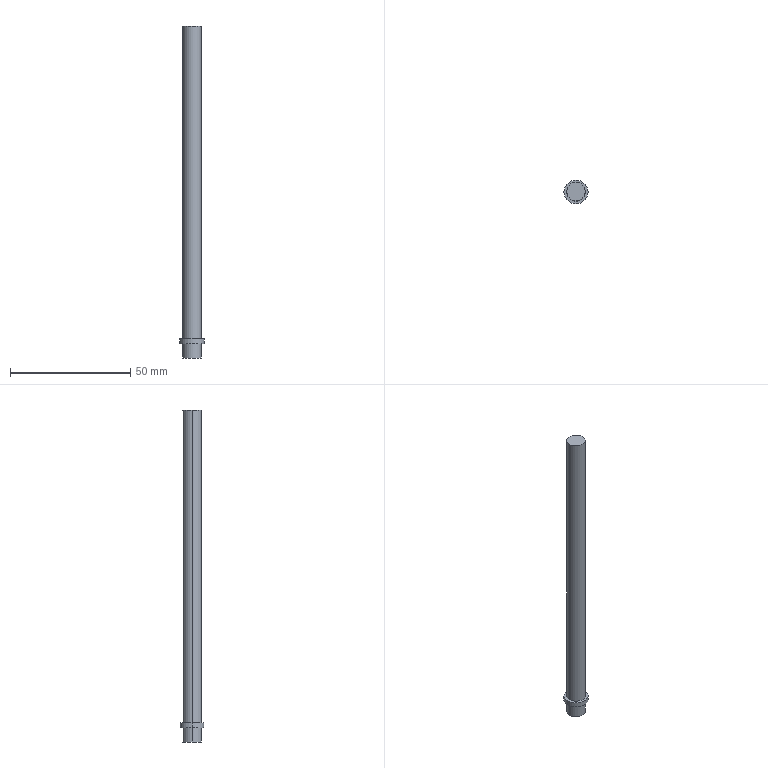Part | SolidWorks | features BaseBody 1 | 1 solid | 10 faces | box 10 x 10 x 138 mm | volume 6490 mm3 | cylinder 6 | plane 4 | commonest cylinder face diameters 7.7 x4 10 x2
STEP:
#1=CARTESIAN_POINT('',(-3.85,0.,-8.));
#2=VERTEX_POINT('',#1);
#3=CARTESIAN_POINT('',(3.85,0.,-8.));
#4=VERTEX_POINT('',#3);
#5=CARTESIAN_POINT('',(0.,0.,-8.));
#6=DIRECTION('',(0.,0.,-1.));
#7=DIRECTION('',(-1.,0.,0.));
#8=AXIS2_PLACEMENT_3D('',#5,#6,#7);
#9=CIRCLE('',#8,3.85);
#10=EDGE_CURVE('',#2,#4,#9,.T.);
#11=ORIENTED_EDGE('',*,*,#10,.F.);
#12=CARTESIAN_POINT('',(-3.85,0.,-2.));
#13=VERTEX_POINT('',#12);
#14=CARTESIAN_POINT('',(-3.85,0.,-8.));
#15=DIRECTION('',(0.,0.,1.));
#16=VECTOR('',#15,1000.);
#17=LINE('',#14,#16);
#18=EDGE_CURVE('',#2,#13,#17,.T.);
#19=ORIENTED_EDGE('',*,*,#18,.T.);
#20=CARTESIAN_POINT('',(3.85,0.,-2.));
#21=VERTEX_POINT('',#20);
#22=CARTESIAN_POINT('',(0.,0.,-2.));
#23=DIRECTION('',(0.,0.,-1.));
#24=DIRECTION('',(-1.,0.,0.));
#25=AXIS2_PLACEMENT_3D('',#22,#23,#24);
#26=CIRCLE('',#25,3.85);
#27=EDGE_CURVE('',#13,#21,#26,.T.);
#28=ORIENTED_EDGE('',*,*,#27,.T.);
#29=CARTESIAN_POINT('',(3.85,0.,-8.));
#30=DIRECTION('',(0.,0.,1.));
#31=VECTOR('',#30,1000.);
#32=LINE('',#29,#31);
#33=EDGE_CURVE('',#4,#21,#32,.T.);
#34=ORIENTED_EDGE('',*,*,#33,.F.);
#35=EDGE_LOOP('',(#11,#19,#28,#34));
#36=FACE_OUTER_BOUND('',#35,.T.);
#37=CARTESIAN_POINT('',(0.,0.,-8.));
#38=DIRECTION('',(0.,0.,1.));
#39=DIRECTION('',(1.,0.,0.));
#40=AXIS2_PLACEMENT_3D('',#37,#38,#39);
#41=CYLINDRICAL_SURFACE('',#40,3.85);
#42=ADVANCED_FACE('',(#36),#41,.T.);
#43=CARTESIAN_POINT('',(-5.,0.,-2.));
#44=VERTEX_POINT('',#43);
#45=CARTESIAN_POINT('',(5.,0.,-2.));
#46=VERTEX_POINT('',#45);
#47=CARTESIAN_POINT('',(0.,0.,-2.));
#48=DIRECTION('',(0.,0.,-1.));
#49=DIRECTION('',(-1.,0.,0.));
#50=AXIS2_PLACEMENT_3D('',#47,#48,#49);
#51=CIRCLE('',#50,5.);
#52=EDGE_CURVE('',#44,#46,#51,.T.);
#53=ORIENTED_EDGE('',*,*,#52,.F.);
#54=CARTESIAN_POINT('',(-5.,0.,0.));
#55=VERTEX_POINT('',#54);
#56=CARTESIAN_POINT('',(-5.,0.,-2.));
#57=DIRECTION('',(0.,0.,1.));
#58=VECTOR('',#57,1000.);
#59=LINE('',#56,#58);
#60=EDGE_CURVE('',#44,#55,#59,.T.);
#61=ORIENTED_EDGE('',*,*,#60,.T.);
#62=CARTESIAN_POINT('',(5.,0.,0.));
#63=VERTEX_POINT('',#62);
#64=CARTESIAN_POINT('',(0.,0.,0.));
#65=DIRECTION('',(0.,0.,-1.));
#66=DIRECTION('',(-1.,0.,0.));
#67=AXIS2_PLACEMENT_3D('',#64,#65,#66);
#68=CIRCLE('',#67,5.);
#69=EDGE_CURVE('',#55,#63,#68,.T.);
#70=ORIENTED_EDGE('',*,*,#69,.T.);
#71=CARTESIAN_POINT('',(5.,0.,-2.));
#72=DIRECTION('',(0.,0.,1.));
#73=VECTOR('',#72,1000.);
#74=LINE('',#71,#73);
#75=EDGE_CURVE('',#46,#63,#74,.T.);
#76=ORIENTED_EDGE('',*,*,#75,.F.);
#77=EDGE_LOOP('',(#53,#61,#70,#76));
#78=FACE_OUTER_BOUND('',#77,.T.);
#79=CARTESIAN_POINT('',(0.,0.,-2.));
#80=DIRECTION('',(0.,0.,1.));
#81=DIRECTION('',(1.,0.,0.));
#82=AXIS2_PLACEMENT_3D('',#79,#80,#81);
#83=CYLINDRICAL_SURFACE('',#82,5.);
#84=ADVANCED_FACE('',(#78),#83,.T.);
#85=CARTESIAN_POINT('',(3.85,0.,130.));
#86=VERTEX_POINT('',#85);
#87=CARTESIAN_POINT('',(-3.85,0.,130.));
#88=VERTEX_POINT('',#87);
#89=CARTESIAN_POINT('',(0.,0.,130.));
#90=DIRECTION('',(0.,0.,1.));
#91=DIRECTION('',(1.,0.,0.));
#92=AXIS2_PLACEMENT_3D('',#89,#90,#91);
#93=CIRCLE('',#92,3.85);
#94=EDGE_CURVE('',#86,#88,#93,.T.);
#95=ORIENTED_EDGE('',*,*,#94,.F.);
#96=CARTESIAN_POINT('',(3.85,0.,0.));
#97=VERTEX_POINT('',#96);
#98=CARTESIAN_POINT('',(3.85,0.,130.));
#99=DIRECTION('',(0.,0.,-1.));
#100=VECTOR('',#99,1000.);
#101=LINE('',#98,#100);
#102=EDGE_CURVE('',#86,#97,#101,.T.);
#103=ORIENTED_EDGE('',*,*,#102,.T.);
#104=CARTESIAN_POINT('',(-3.85,0.,0.));
#105=VERTEX_POINT('',#104);
#106=CARTESIAN_POINT('',(0.,0.,0.));
#107=DIRECTION('',(0.,0.,1.));
#108=DIRECTION('',(1.,0.,0.));
#109=AXIS2_PLACEMENT_3D('',#106,#107,#108);
#110=CIRCLE('',#109,3.85);
#111=EDGE_CURVE('',#97,#105,#110,.T.);
#112=ORIENTED_EDGE('',*,*,#111,.T.);
#113=CARTESIAN_POINT('',(-3.85,0.,130.));
#114=DIRECTION('',(0.,0.,-1.));
#115=VECTOR('',#114,1000.);
#116=LINE('',#113,#115);
#117=EDGE_CURVE('',#88,#105,#116,.T.);
#118=ORIENTED_EDGE('',*,*,#117,.F.);
#119=EDGE_LOOP('',(#95,#103,#112,#118));
#120=FACE_OUTER_BOUND('',#119,.T.);
#121=CARTESIAN_POINT('',(0.,0.,130.));
#122=DIRECTION('',(0.,0.,-1.));
#123=DIRECTION('',(-1.,0.,0.));
#124=AXIS2_PLACEMENT_3D('',#121,#122,#123);
#125=CYLINDRICAL_SURFACE('',#124,3.85);
#126=ADVANCED_FACE('',(#120),#125,.T.);
#127=CARTESIAN_POINT('',(0.,0.,-8.));
#128=DIRECTION('',(0.,0.,-1.));
#129=DIRECTION('',(-1.,0.,0.));
#130=AXIS2_PLACEMENT_3D('',#127,#128,#129);
#131=CIRCLE('',#130,3.85);
#132=EDGE_CURVE('',#4,#2,#131,.T.);
#133=ORIENTED_EDGE('',*,*,#132,.T.);
#134=ORIENTED_EDGE('',*,*,#10,.T.);
#135=EDGE_LOOP('',(#133,#134));
#136=FACE_OUTER_BOUND('',#135,.T.);
#137=CARTESIAN_POINT('',(0.,0.,-8.));
#138=DIRECTION('',(0.,0.,-1.));
#139=DIRECTION('',(0.,-1.,0.));
#140=AXIS2_PLACEMENT_3D('',#137,#138,#139);
#141=PLANE('',#140);
#142=ADVANCED_FACE('',(#136),#141,.T.);
#143=CARTESIAN_POINT('',(0.,0.,0.));
#144=DIRECTION('',(0.,0.,1.));
#145=DIRECTION('',(1.,0.,0.));
#146=AXIS2_PLACEMENT_3D('',#143,#144,#145);
#147=CIRCLE('',#146,3.85);
#148=EDGE_CURVE('',#105,#97,#147,.T.);
#149=ORIENTED_EDGE('',*,*,#148,.F.);
#150=ORIENTED_EDGE('',*,*,#111,.F.);
#151=EDGE_LOOP('',(#149,#150));
#152=FACE_BOUND('',#151,.T.);
#153=CARTESIAN_POINT('',(0.,0.,0.));
#154=DIRECTION('',(0.,0.,-1.));
#155=DIRECTION('',(-1.,0.,0.));
#156=AXIS2_PLACEMENT_3D('',#153,#154,#155);
#157=CIRCLE('',#156,5.);
#158=EDGE_CURVE('',#63,#55,#157,.T.);
#159=ORIENTED_EDGE('',*,*,#158,.F.);
#160=ORIENTED_EDGE('',*,*,#69,.F.);
#161=EDGE_LOOP('',(#159,#160));
#162=FACE_OUTER_BOUND('',#161,.T.);
#163=CARTESIAN_POINT('',(0.,0.,0.));
#164=DIRECTION('',(0.,0.,-1.));
#165=DIRECTION('',(0.,-1.,0.));
#166=AXIS2_PLACEMENT_3D('',#163,#164,#165);
#167=PLANE('',#166);
#168=ADVANCED_FACE('',(#152,#162),#167,.F.);
#169=CARTESIAN_POINT('',(0.,0.,-2.));
#170=DIRECTION('',(0.,0.,-1.));
#171=DIRECTION('',(-1.,0.,0.));
#172=AXIS2_PLACEMENT_3D('',#169,#170,#171);
#173=CIRCLE('',#172,3.85);
#174=EDGE_CURVE('',#21,#13,#173,.T.);
#175=ORIENTED_EDGE('',*,*,#174,.F.);
#176=ORIENTED_EDGE('',*,*,#27,.F.);
#177=EDGE_LOOP('',(#175,#176));
#178=FACE_BOUND('',#177,.T.);
#179=CARTESIAN_POINT('',(0.,0.,-2.));
#180=DIRECTION('',(0.,0.,-1.));
#181=DIRECTION('',(-1.,0.,0.));
#182=AXIS2_PLACEMENT_3D('',#179,#180,#181);
#183=CIRCLE('',#182,5.);
#184=EDGE_CURVE('',#46,#44,#183,.T.);
#185=ORIENTED_EDGE('',*,*,#184,.T.);
#186=ORIENTED_EDGE('',*,*,#52,.T.);
#187=EDGE_LOOP('',(#185,#186));
#188=FACE_OUTER_BOUND('',#187,.T.);
#189=CARTESIAN_POINT('',(0.,0.,-2.));
#190=DIRECTION('',(0.,0.,-1.));
#191=DIRECTION('',(0.,-1.,0.));
#192=AXIS2_PLACEMENT_3D('',#189,#190,#191);
#193=PLANE('',#192);
#194=ADVANCED_FACE('',(#178,#188),#193,.T.);
#195=CARTESIAN_POINT('',(0.,0.,130.));
#196=DIRECTION('',(0.,0.,1.));
#197=DIRECTION('',(1.,0.,0.));
#198=AXIS2_PLACEMENT_3D('',#195,#196,#197);
#199=CIRCLE('',#198,3.85);
#200=EDGE_CURVE('',#88,#86,#199,.T.);
#201=ORIENTED_EDGE('',*,*,#200,.T.);
#202=ORIENTED_EDGE('',*,*,#94,.T.);
#203=EDGE_LOOP('',(#201,#202));
#204=FACE_OUTER_BOUND('',#203,.T.);
#205=CARTESIAN_POINT('',(0.,0.,130.));
#206=DIRECTION('',(0.,0.,1.));
#207=DIRECTION('',(1.,0.,0.));
#208=AXIS2_PLACEMENT_3D('',#205,#206,#207);
#209=PLANE('',#208);
#210=ADVANCED_FACE('',(#204),#209,.T.);
#211=ORIENTED_EDGE('',*,*,#102,.F.);
#212=ORIENTED_EDGE('',*,*,#200,.F.);
#213=ORIENTED_EDGE('',*,*,#117,.T.);
#214=ORIENTED_EDGE('',*,*,#148,.T.);
#215=EDGE_LOOP('',(#211,#212,#213,#214));
#216=FACE_OUTER_BOUND('',#215,.T.);
#217=CARTESIAN_POINT('',(0.,0.,130.));
#218=DIRECTION('',(0.,0.,-1.));
#219=DIRECTION('',(-1.,0.,0.));
#220=AXIS2_PLACEMENT_3D('',#217,#218,#219);
#221=CYLINDRICAL_SURFACE('',#220,3.85);
#222=ADVANCED_FACE('',(#216),#221,.T.);
#223=ORIENTED_EDGE('',*,*,#60,.F.);
#224=ORIENTED_EDGE('',*,*,#184,.F.);
#225=ORIENTED_EDGE('',*,*,#75,.T.);
#226=ORIENTED_EDGE('',*,*,#158,.T.);
#227=EDGE_LOOP('',(#223,#224,#225,#226));
#228=FACE_OUTER_BOUND('',#227,.T.);
#229=CARTESIAN_POINT('',(0.,0.,-2.));
#230=DIRECTION('',(0.,0.,1.));
#231=DIRECTION('',(1.,0.,0.));
#232=AXIS2_PLACEMENT_3D('',#229,#230,#231);
#233=CYLINDRICAL_SURFACE('',#232,5.);
#234=ADVANCED_FACE('',(#228),#233,.T.);
#235=ORIENTED_EDGE('',*,*,#18,.F.);
#236=ORIENTED_EDGE('',*,*,#132,.F.);
#237=ORIENTED_EDGE('',*,*,#33,.T.);
#238=ORIENTED_EDGE('',*,*,#174,.T.);
#239=EDGE_LOOP('',(#235,#236,#237,#238));
#240=FACE_OUTER_BOUND('',#239,.T.);
#241=CARTESIAN_POINT('',(0.,0.,-8.));
#242=DIRECTION('',(0.,0.,1.));
#243=DIRECTION('',(1.,0.,0.));
#244=AXIS2_PLACEMENT_3D('',#241,#242,#243);
#245=CYLINDRICAL_SURFACE('',#244,3.85);
#246=ADVANCED_FACE('',(#240),#245,.T.);
#247=CLOSED_SHELL('',(#42,#84,#126,#142,#168,#194,#210,#222,#234,#246));
#248=MANIFOLD_SOLID_BREP('',#247);
#249=CARTESIAN_POINT('',(0.,0.,0.));
#250=DIRECTION('',(0.,0.,1.));
#251=DIRECTION('',(1.,0.,0.));
#252=AXIS2_PLACEMENT_3D('',#249,#250,#251);
#253=(LENGTH_UNIT()NAMED_UNIT(*)SI_UNIT(.MILLI.,.METRE.));
#254=UNCERTAINTY_MEASURE_WITH_UNIT(LENGTH_MEASURE(0.00001),#253,'','');
#255=(NAMED_UNIT(*)PLANE_ANGLE_UNIT()SI_UNIT($,.RADIAN.));
#256=(NAMED_UNIT(*)SI_UNIT($,.STERADIAN.)SOLID_ANGLE_UNIT());
#257=(GEOMETRIC_REPRESENTATION_CONTEXT(3)GLOBAL_UNCERTAINTY_ASSIGNED_CONTEXT((#254))GLOBAL_UNIT_ASSIGNED_CONTEXT((#253,#255,#256))REPRESENTATION_CONTEXT('',''));
#258=ADVANCED_BREP_SHAPE_REPRESENTATION('',(#248,#252),#257);